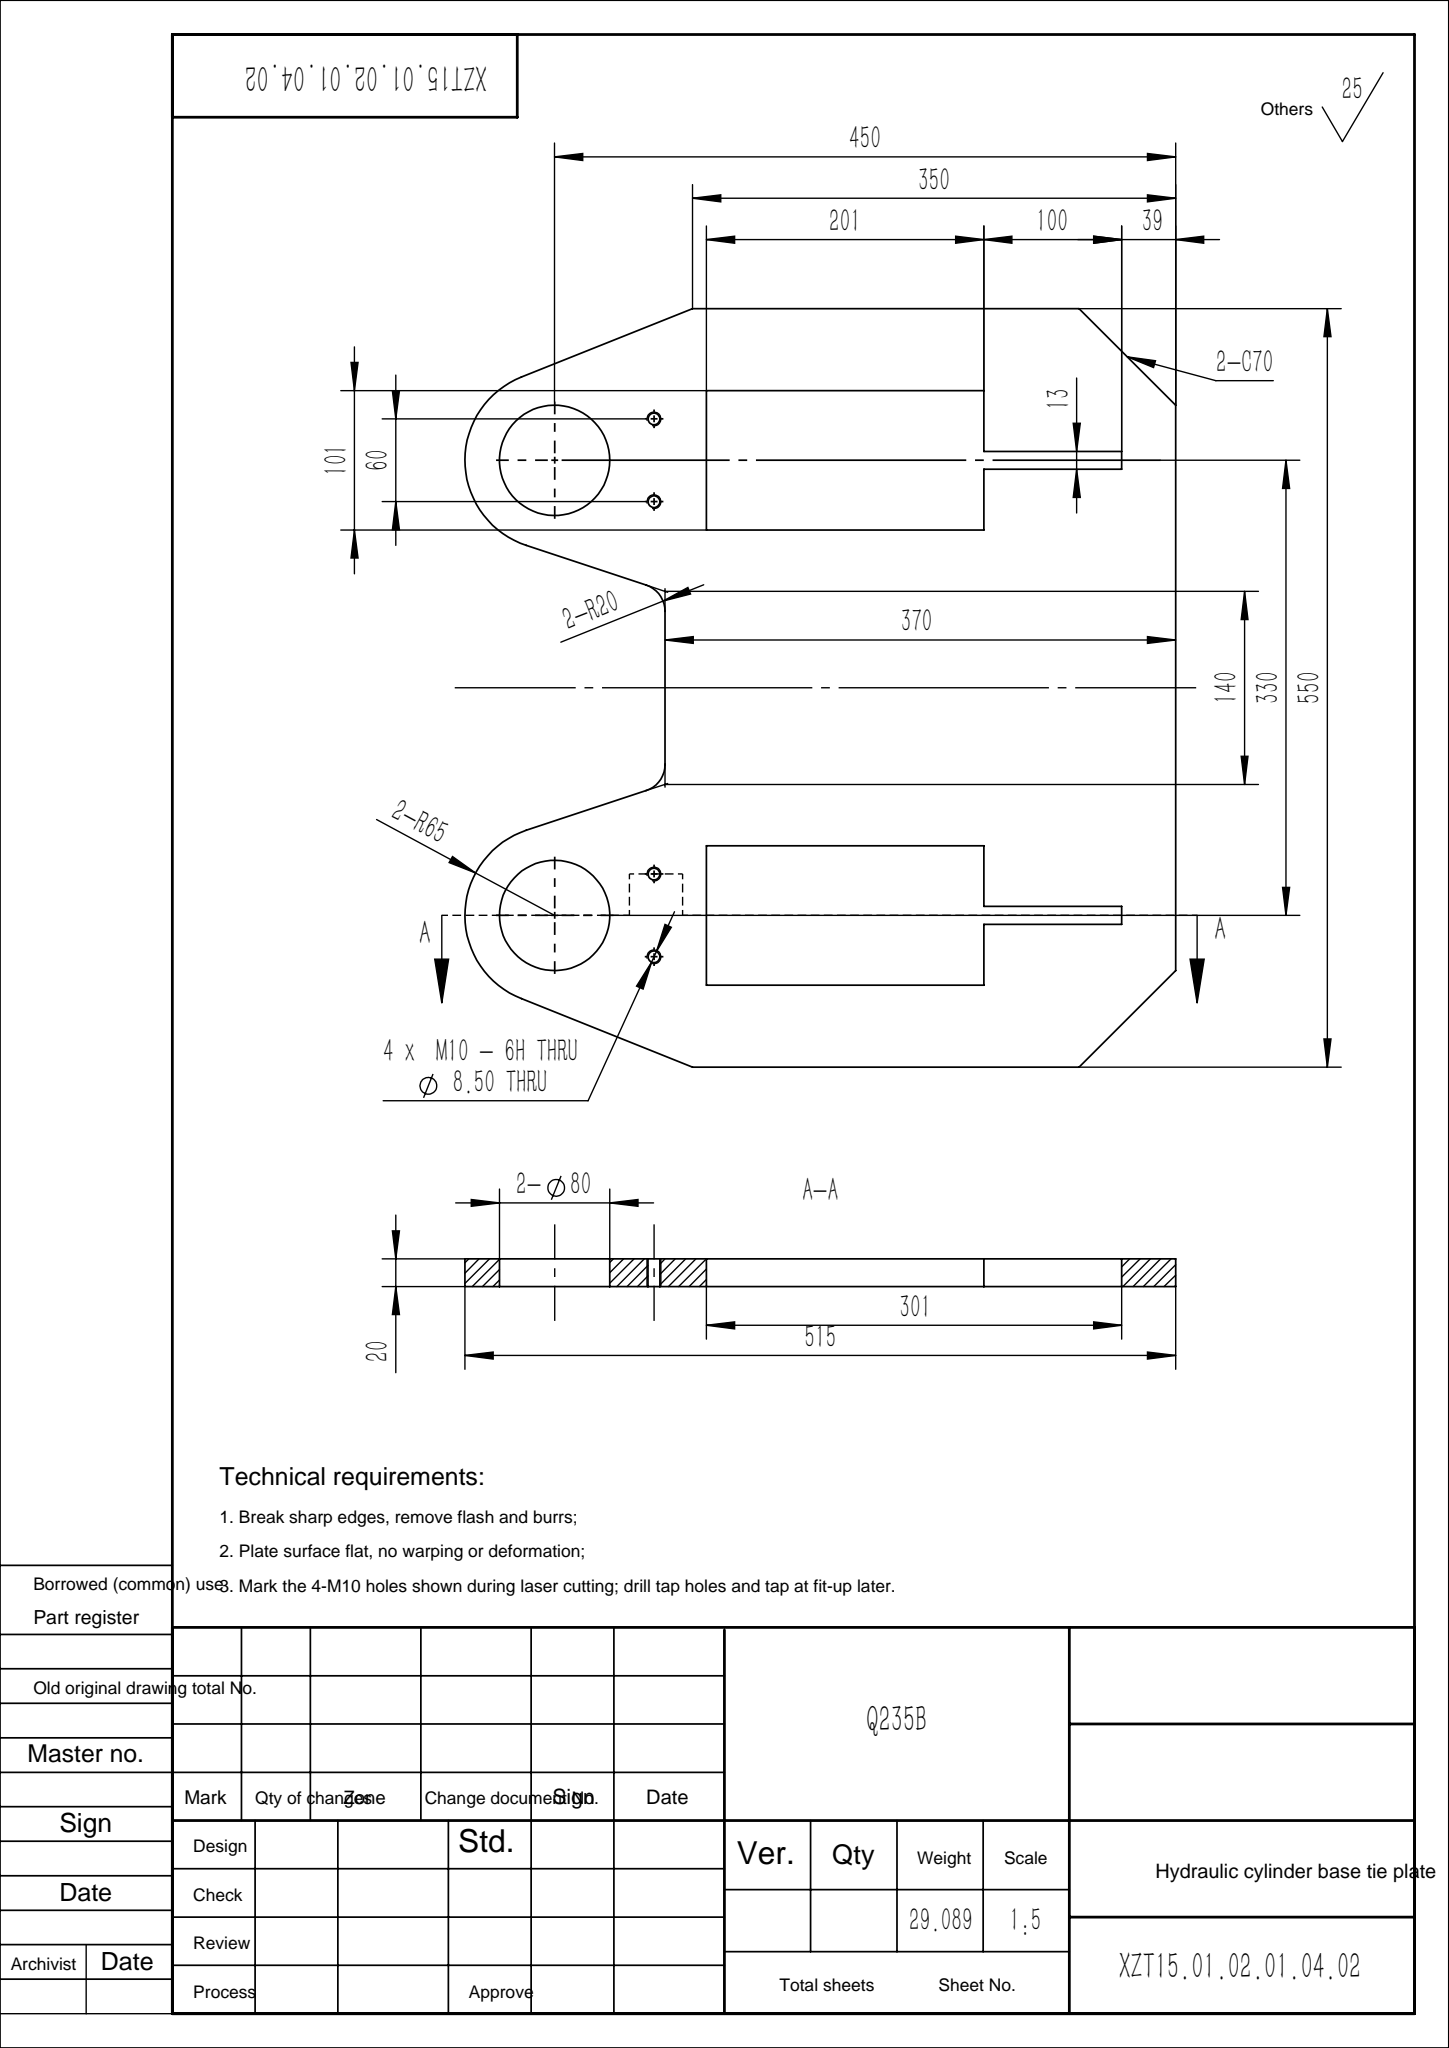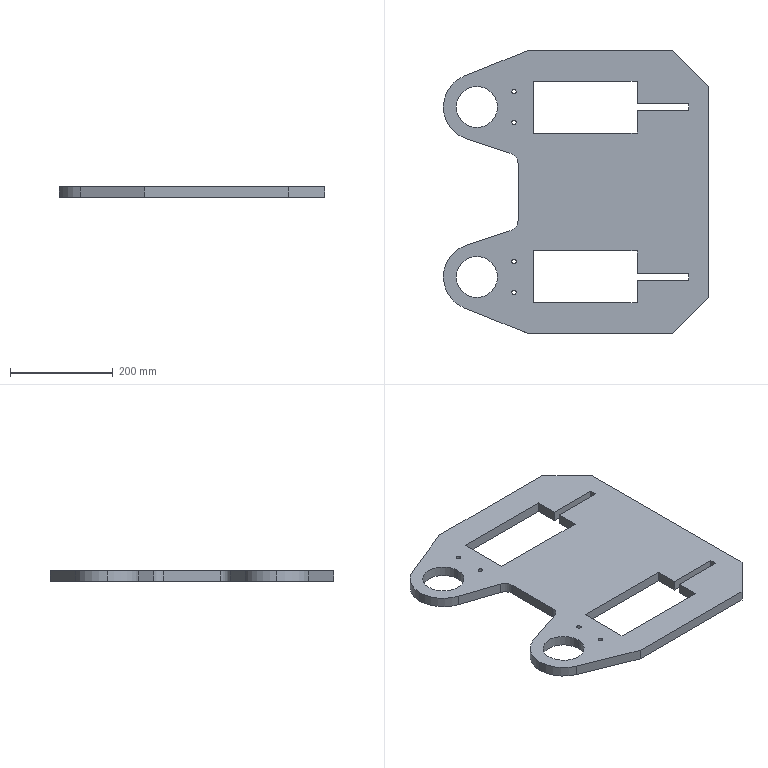Part | SolidWorks | features Chamfer 1, Extrusion 1, Fillet 1, HoleWzd 1 | 1 solid | 46 faces | box 515 x 550 x 20 mm | volume 3705557 mm3 | plane 28 | cylinder 18 | commonest cylinder face diameters 8.5 x8 80 x4 130 x4 40 x2